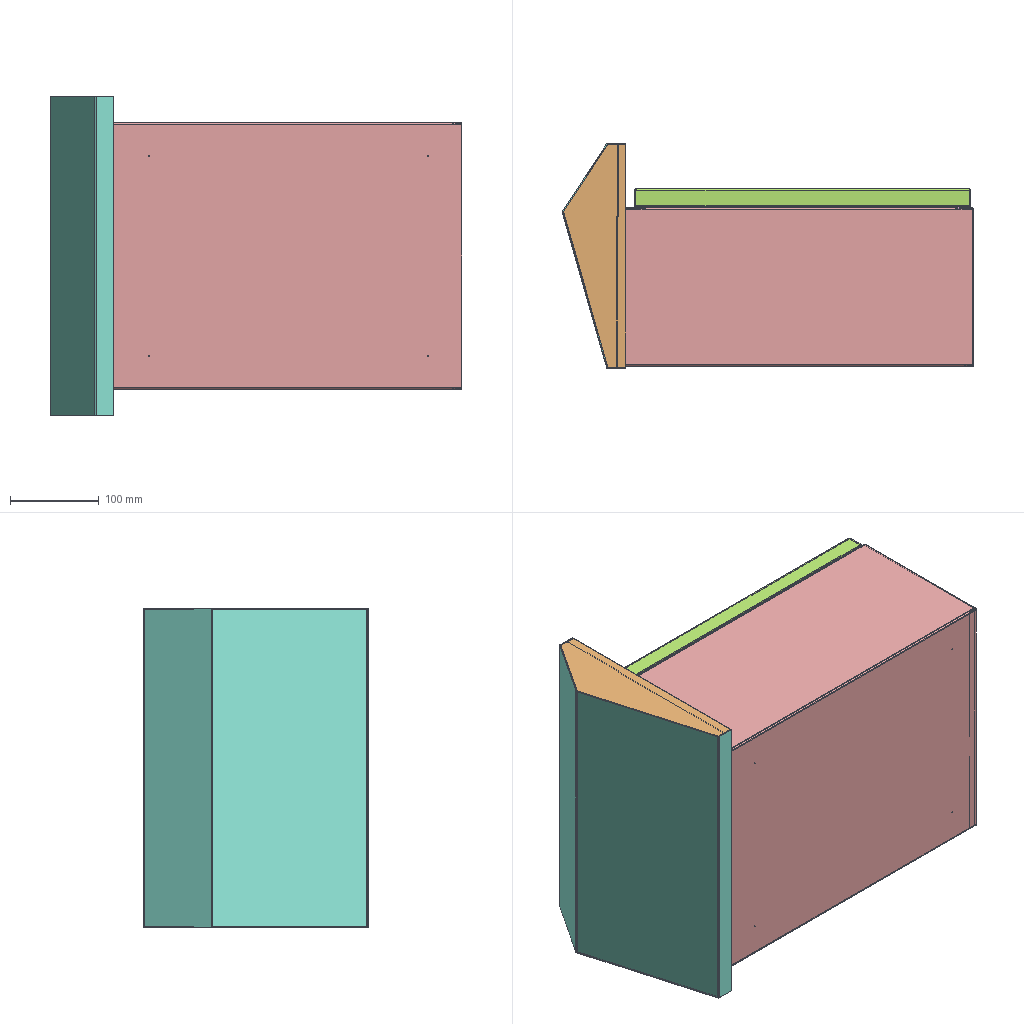Assembly | SolidWorks | 14 different items | 14 placed | box 463 x 254 x 360 mm
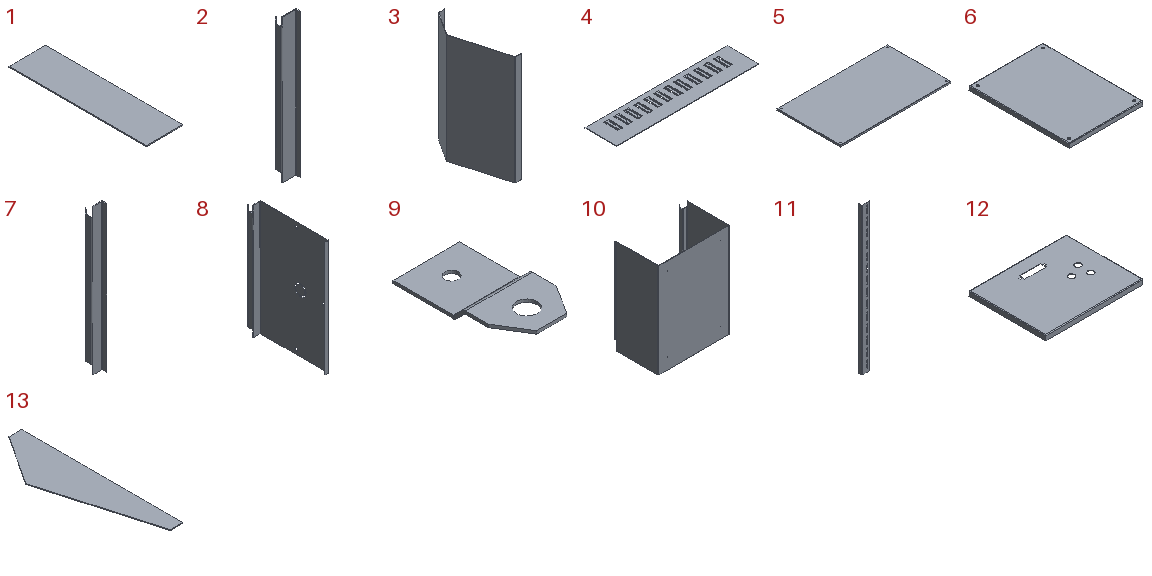Parts list (item | name | quantity | size | volume | features):
1 | - | x1 | 45 x 168.6 x 1.2 mm | 9104 mm3 | features FlatPattern 1, SMBaseFlange 1, SheetMetal 1
2 | - | x1 | 30.2 x 28.771 x 297.6 mm | 19971 mm3 | features SMBaseFlange 2, Cut 1, FlatPattern 1, MirrorPattern 1, SheetMetal 1
3 | - | x1 | 71.113 x 253.6 x 360 mm | 135935 mm3 | features FlatPattern 1, SMBaseFlange 1, SheetMetal 1
4 | - | x1 | 357.6 x 80 x 4.201 mm | 34630 mm3 | features FlatPattern 1, FormToolInstance 1, LPattern 1, SMBaseFlange 1, SheetMetal 1
5 | - | x1 | 907 x 520 x 13.8 mm | 606294 mm3 | features 3DProfileFeature 1, EdgeFlange 1, FlatPattern 1, HoleWzd 1, SMBaseFlange 1, SheetMetal 1
6 | - | x1 | 254.629 x 344.629 x 15 mm | 123831 mm3 | features CornerFeat 1, Cut 1, EdgeFlange 1, FlatPattern 1, MoveCopyBody 1, SMBaseFlange 1, SheetMetal 1
7 | - | x1 | 22.2 x 28.771 x 297.6 mm | 16962 mm3 | features CombineBodies 1, FlatPattern 1, FlattenBends 1, ICE 1, MirrorStock 1, MoveCopyBody 1, ProcessBends 1, SheetMetal 1
8 | - | x1 | 20.2 x 196.571 x 297.6 mm | 78731 mm3 | features Attribute 55, Cut 2, SMBaseFlange 2, FlatPattern 1, ICE 1, LibraryFeature 1, MirrorPattern 1, SheetMetal 1
9 | - | x1 | 40 x 75 x 7.8 mm | 4907 mm3 | features FlatPattern 1, Jog 1, SMBaseFlange 1, SheetMetal 1
10 | - | x1 | 300 x 197.771 x 400 mm | 345884 mm3 | features Cut 3, FlatPattern 1, SMBaseFlange 1, SheetMetal 1
11 | - | x1 | 50 x 25 x 997.6 mm | 119077 mm3 | features BaseBody 1
12 | - | x1 | 378.8 x 297.75 x 19.5 mm | 199133 mm3 | features Cut 3, CornerFeat 1, EdgeFlange 1, FlatPattern 1, ICE 1, LPattern 1, LibraryFeature 1, SMBaseFlange 1, SheetMetal 1
13 | - | x1 | 69.783 x 250.8 x 1.2 mm | 13490 mm3 | features FlatPattern 1, SMBaseFlange 1, SheetMetal 1
14 | countersunk head rivets--black gb | x1 | - | - | -
Mates (type | each side: item.copy, entity, surface, feature):
InPlace | 10.1 plane | assembly plane
InPlace | 10.1 face plane Base-Flange 1 | 2.1 plane
InPlace | 12.1 plane | assembly plane
InPlace | 10.1 face plane Base-Flange 1 | 8.1 plane
InPlace | 3.1 plane | assembly plane
InPlace | 3.1 face plane Base-Flange 1 | 13.1 plane
InPlace | 2.1 face plane Base-Flange 1 | 4.1 plane
InPlace | 4.1 face plane Base-Flange 1 | 1.1 plane
InPlace | 10.1 face plane Base-Flange 1 | 6.1 plane